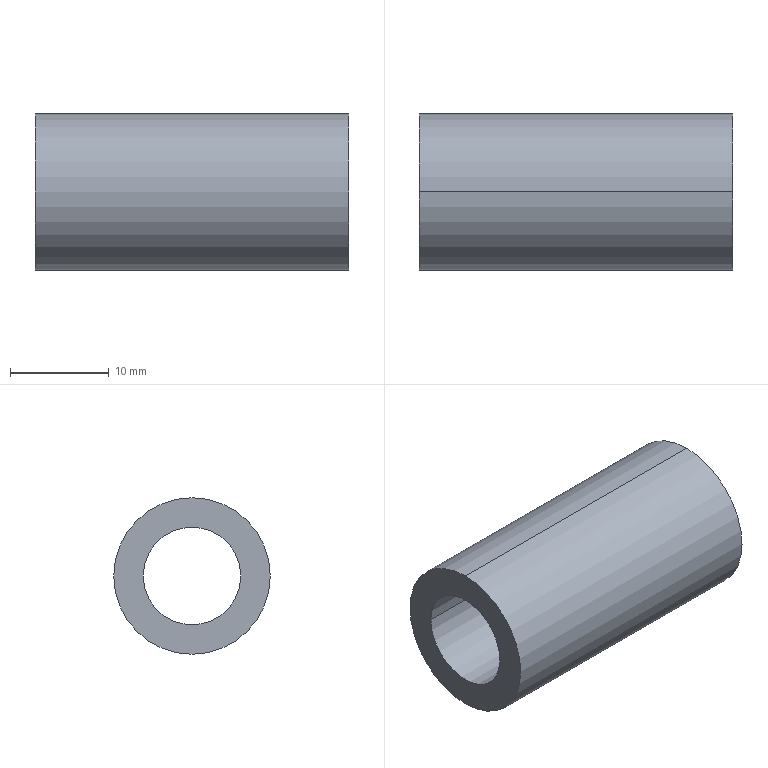Part | NX | features BREP 1 | 1 solid | 6 faces | box 31.75 x 15.875 x 15.875 mm | volume 3837 mm3 | cylinder 4 | plane 2 | commonest cylinder face diameters 9.906 x2 15.875 x2
STEP:
#1=CARTESIAN_POINT('',(0.,0.,7.938));
#2=VERTEX_POINT('',#1);
#3=CARTESIAN_POINT('',(0.,0.,-7.938));
#4=VERTEX_POINT('',#3);
#5=CARTESIAN_POINT('',(0.,0.,0.));
#6=DIRECTION('',(1.,0.,0.));
#7=DIRECTION('',(0.,0.,1.));
#8=AXIS2_PLACEMENT_3D('',#5,#6,#7);
#9=CIRCLE('',#8,7.938);
#10=EDGE_CURVE('',#2,#4,#9,.T.);
#11=ORIENTED_EDGE('',*,*,#10,.F.);
#12=CARTESIAN_POINT('',(0.,0.,0.));
#13=DIRECTION('',(1.,0.,0.));
#14=DIRECTION('',(0.,0.,-1.));
#15=AXIS2_PLACEMENT_3D('',#12,#13,#14);
#16=CIRCLE('',#15,7.938);
#17=EDGE_CURVE('',#4,#2,#16,.T.);
#18=ORIENTED_EDGE('',*,*,#17,.F.);
#19=EDGE_LOOP('',(#11,#18));
#20=FACE_BOUND('',#19,.T.);
#21=CARTESIAN_POINT('',(0.,-4.953,0.));
#22=VERTEX_POINT('',#21);
#23=CARTESIAN_POINT('',(0.,4.953,0.));
#24=VERTEX_POINT('',#23);
#25=CARTESIAN_POINT('',(0.,0.,0.));
#26=DIRECTION('',(1.,0.,0.));
#27=DIRECTION('',(0.,-1.,0.));
#28=AXIS2_PLACEMENT_3D('',#25,#26,#27);
#29=CIRCLE('',#28,4.953);
#30=EDGE_CURVE('',#22,#24,#29,.T.);
#31=ORIENTED_EDGE('',*,*,#30,.T.);
#32=CARTESIAN_POINT('',(0.,0.,0.));
#33=DIRECTION('',(1.,0.,0.));
#34=DIRECTION('',(0.,1.,0.));
#35=AXIS2_PLACEMENT_3D('',#32,#33,#34);
#36=CIRCLE('',#35,4.953);
#37=EDGE_CURVE('',#24,#22,#36,.T.);
#38=ORIENTED_EDGE('',*,*,#37,.T.);
#39=EDGE_LOOP('',(#31,#38));
#40=FACE_BOUND('',#39,.T.);
#41=CARTESIAN_POINT('',(0.,0.,0.));
#42=DIRECTION('',(1.,0.,0.));
#43=DIRECTION('',(0.,1.,0.));
#44=AXIS2_PLACEMENT_3D('',#41,#42,#43);
#45=PLANE('',#44);
#46=ADVANCED_FACE('',(#20,#40),#45,.F.);
#47=CARTESIAN_POINT('',(31.75,0.,7.938));
#48=VERTEX_POINT('',#47);
#49=CARTESIAN_POINT('',(0.,0.,7.938));
#50=DIRECTION('',(1.,0.,0.));
#51=VECTOR('',#50,1000.);
#52=LINE('',#49,#51);
#53=EDGE_CURVE('',#48,#2,#52,.F.);
#54=ORIENTED_EDGE('',*,*,#53,.F.);
#55=CARTESIAN_POINT('',(31.75,0.,-7.938));
#56=VERTEX_POINT('',#55);
#57=CARTESIAN_POINT('',(31.75,0.,0.));
#58=DIRECTION('',(1.,0.,0.));
#59=DIRECTION('',(0.,0.,-1.));
#60=AXIS2_PLACEMENT_3D('',#57,#58,#59);
#61=CIRCLE('',#60,7.938);
#62=EDGE_CURVE('',#56,#48,#61,.T.);
#63=ORIENTED_EDGE('',*,*,#62,.F.);
#64=CARTESIAN_POINT('',(0.,0.,-7.938));
#65=DIRECTION('',(1.,0.,0.));
#66=VECTOR('',#65,1000.);
#67=LINE('',#64,#66);
#68=EDGE_CURVE('',#56,#4,#67,.F.);
#69=ORIENTED_EDGE('',*,*,#68,.T.);
#70=ORIENTED_EDGE('',*,*,#17,.T.);
#71=EDGE_LOOP('',(#54,#63,#69,#70));
#72=FACE_BOUND('',#71,.T.);
#73=CARTESIAN_POINT('',(0.,0.,0.));
#74=DIRECTION('',(1.,0.,0.));
#75=DIRECTION('',(0.,0.,-1.));
#76=AXIS2_PLACEMENT_3D('',#73,#74,#75);
#77=CYLINDRICAL_SURFACE('',#76,7.938);
#78=ADVANCED_FACE('',(#72),#77,.T.);
#79=ORIENTED_EDGE('',*,*,#68,.F.);
#80=CARTESIAN_POINT('',(31.75,0.,0.));
#81=DIRECTION('',(1.,0.,0.));
#82=DIRECTION('',(0.,0.,1.));
#83=AXIS2_PLACEMENT_3D('',#80,#81,#82);
#84=CIRCLE('',#83,7.938);
#85=EDGE_CURVE('',#48,#56,#84,.T.);
#86=ORIENTED_EDGE('',*,*,#85,.F.);
#87=ORIENTED_EDGE('',*,*,#53,.T.);
#88=ORIENTED_EDGE('',*,*,#10,.T.);
#89=EDGE_LOOP('',(#79,#86,#87,#88));
#90=FACE_BOUND('',#89,.T.);
#91=CARTESIAN_POINT('',(0.,0.,0.));
#92=DIRECTION('',(1.,0.,0.));
#93=DIRECTION('',(0.,0.,-1.));
#94=AXIS2_PLACEMENT_3D('',#91,#92,#93);
#95=CYLINDRICAL_SURFACE('',#94,7.938);
#96=ADVANCED_FACE('',(#90),#95,.T.);
#97=ORIENTED_EDGE('',*,*,#85,.T.);
#98=ORIENTED_EDGE('',*,*,#62,.T.);
#99=EDGE_LOOP('',(#97,#98));
#100=FACE_BOUND('',#99,.T.);
#101=CARTESIAN_POINT('',(31.75,-4.953,0.));
#102=VERTEX_POINT('',#101);
#103=CARTESIAN_POINT('',(31.75,4.953,0.));
#104=VERTEX_POINT('',#103);
#105=CARTESIAN_POINT('',(31.75,0.,0.));
#106=DIRECTION('',(1.,0.,0.));
#107=DIRECTION('',(0.,-1.,0.));
#108=AXIS2_PLACEMENT_3D('',#105,#106,#107);
#109=CIRCLE('',#108,4.953);
#110=EDGE_CURVE('',#102,#104,#109,.T.);
#111=ORIENTED_EDGE('',*,*,#110,.F.);
#112=CARTESIAN_POINT('',(31.75,0.,0.));
#113=DIRECTION('',(1.,0.,0.));
#114=DIRECTION('',(0.,1.,0.));
#115=AXIS2_PLACEMENT_3D('',#112,#113,#114);
#116=CIRCLE('',#115,4.953);
#117=EDGE_CURVE('',#104,#102,#116,.T.);
#118=ORIENTED_EDGE('',*,*,#117,.F.);
#119=EDGE_LOOP('',(#111,#118));
#120=FACE_BOUND('',#119,.T.);
#121=CARTESIAN_POINT('',(31.75,0.,0.));
#122=DIRECTION('',(1.,0.,0.));
#123=DIRECTION('',(0.,1.,0.));
#124=AXIS2_PLACEMENT_3D('',#121,#122,#123);
#125=PLANE('',#124);
#126=ADVANCED_FACE('',(#100,#120),#125,.T.);
#127=CARTESIAN_POINT('',(0.,4.953,0.));
#128=DIRECTION('',(1.,0.,0.));
#129=VECTOR('',#128,1000.);
#130=LINE('',#127,#129);
#131=EDGE_CURVE('',#104,#24,#130,.F.);
#132=ORIENTED_EDGE('',*,*,#131,.F.);
#133=ORIENTED_EDGE('',*,*,#117,.T.);
#134=CARTESIAN_POINT('',(0.,-4.953,0.));
#135=DIRECTION('',(1.,0.,0.));
#136=VECTOR('',#135,1000.);
#137=LINE('',#134,#136);
#138=EDGE_CURVE('',#102,#22,#137,.F.);
#139=ORIENTED_EDGE('',*,*,#138,.T.);
#140=ORIENTED_EDGE('',*,*,#37,.F.);
#141=EDGE_LOOP('',(#132,#133,#139,#140));
#142=FACE_BOUND('',#141,.T.);
#143=CARTESIAN_POINT('',(0.,0.,0.));
#144=DIRECTION('',(1.,0.,0.));
#145=DIRECTION('',(0.,1.,0.));
#146=AXIS2_PLACEMENT_3D('',#143,#144,#145);
#147=CYLINDRICAL_SURFACE('',#146,4.953);
#148=ADVANCED_FACE('',(#142),#147,.F.);
#149=ORIENTED_EDGE('',*,*,#138,.F.);
#150=ORIENTED_EDGE('',*,*,#110,.T.);
#151=ORIENTED_EDGE('',*,*,#131,.T.);
#152=ORIENTED_EDGE('',*,*,#30,.F.);
#153=EDGE_LOOP('',(#149,#150,#151,#152));
#154=FACE_BOUND('',#153,.T.);
#155=CARTESIAN_POINT('',(0.,0.,0.));
#156=DIRECTION('',(1.,0.,0.));
#157=DIRECTION('',(0.,1.,0.));
#158=AXIS2_PLACEMENT_3D('',#155,#156,#157);
#159=CYLINDRICAL_SURFACE('',#158,4.953);
#160=ADVANCED_FACE('',(#154),#159,.F.);
#161=CLOSED_SHELL('',(#46,#78,#96,#126,#148,#160));
#162=MANIFOLD_SOLID_BREP('',#161);
#163=(LENGTH_UNIT()NAMED_UNIT(*)SI_UNIT(.MILLI.,.METRE.));
#164=UNCERTAINTY_MEASURE_WITH_UNIT(LENGTH_MEASURE(0.00001),#163,'','');
#165=(NAMED_UNIT(*)PLANE_ANGLE_UNIT()SI_UNIT($,.RADIAN.));
#166=(NAMED_UNIT(*)SI_UNIT($,.STERADIAN.)SOLID_ANGLE_UNIT());
#167=(GEOMETRIC_REPRESENTATION_CONTEXT(3)GLOBAL_UNCERTAINTY_ASSIGNED_CONTEXT((#164))GLOBAL_UNIT_ASSIGNED_CONTEXT((#163,#165,#166))REPRESENTATION_CONTEXT('',''));
#168=ADVANCED_BREP_SHAPE_REPRESENTATION('',(#162),#167);